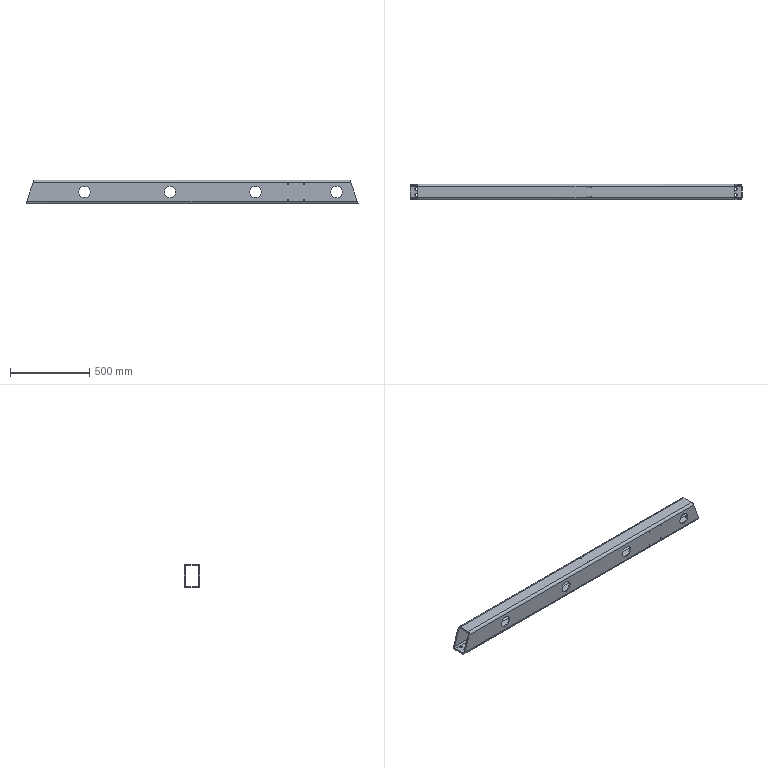Part | STEP file | 011-Rectangular tube 150x100x8_default<machining> | 1 solid | 58 faces | box 2098 x 100 x 150 mm | volume 7060017 mm3 | cylinder 48 | plane 10 | commonest cylinder face diameters 72 x16 3.3 x8 6.8 x8 18 x8 16 x4 32 x4